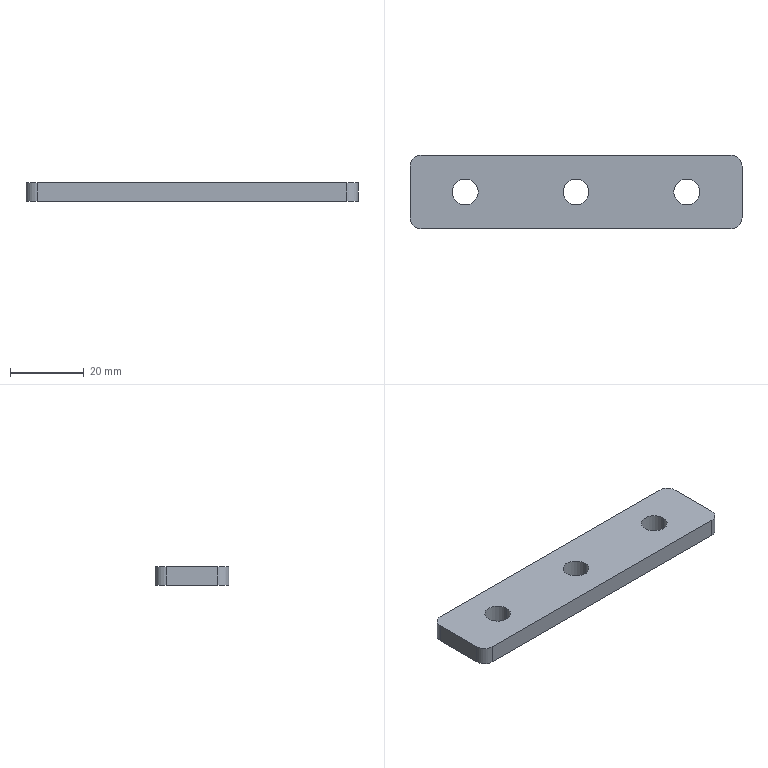Part | SolidWorks | features BaseBody 1 | 1 solid | 16 faces | box 90 x 20 x 5 mm | volume 8384 mm3 | cylinder 10 | plane 6 | commonest cylinder face diameters 7 x6 6 x4
STEP:
#1=CARTESIAN_POINT('',(26.5,0.,5.));
#2=VERTEX_POINT('',#1);
#3=CARTESIAN_POINT('',(33.5,0.,5.));
#4=VERTEX_POINT('',#3);
#5=CARTESIAN_POINT('',(30.,0.,5.));
#6=DIRECTION('',(0.,0.,1.));
#7=DIRECTION('',(1.,0.,0.));
#8=AXIS2_PLACEMENT_3D('',#5,#6,#7);
#9=CIRCLE('',#8,3.5);
#10=EDGE_CURVE('',#2,#4,#9,.T.);
#11=ORIENTED_EDGE('',*,*,#10,.T.);
#12=CARTESIAN_POINT('',(33.5,0.,0.));
#13=VERTEX_POINT('',#12);
#14=CARTESIAN_POINT('',(33.5,0.,5.));
#15=DIRECTION('',(0.,0.,-1.));
#16=VECTOR('',#15,1000.);
#17=LINE('',#14,#16);
#18=EDGE_CURVE('',#4,#13,#17,.T.);
#19=ORIENTED_EDGE('',*,*,#18,.T.);
#20=CARTESIAN_POINT('',(26.5,0.,0.));
#21=VERTEX_POINT('',#20);
#22=CARTESIAN_POINT('',(30.,0.,0.));
#23=DIRECTION('',(0.,0.,1.));
#24=DIRECTION('',(1.,0.,0.));
#25=AXIS2_PLACEMENT_3D('',#22,#23,#24);
#26=CIRCLE('',#25,3.5);
#27=EDGE_CURVE('',#21,#13,#26,.T.);
#28=ORIENTED_EDGE('',*,*,#27,.F.);
#29=CARTESIAN_POINT('',(26.5,0.,5.));
#30=DIRECTION('',(0.,0.,-1.));
#31=VECTOR('',#30,1000.);
#32=LINE('',#29,#31);
#33=EDGE_CURVE('',#2,#21,#32,.T.);
#34=ORIENTED_EDGE('',*,*,#33,.F.);
#35=EDGE_LOOP('',(#11,#19,#28,#34));
#36=FACE_OUTER_BOUND('',#35,.T.);
#37=CARTESIAN_POINT('',(30.,0.,5.));
#38=DIRECTION('',(0.,0.,-1.));
#39=DIRECTION('',(-1.,0.,0.));
#40=AXIS2_PLACEMENT_3D('',#37,#38,#39);
#41=CYLINDRICAL_SURFACE('',#40,3.5);
#42=ADVANCED_FACE('',(#36),#41,.F.);
#43=CARTESIAN_POINT('',(-3.5,0.,5.));
#44=VERTEX_POINT('',#43);
#45=CARTESIAN_POINT('',(3.5,0.,5.));
#46=VERTEX_POINT('',#45);
#47=CARTESIAN_POINT('',(0.,0.,5.));
#48=DIRECTION('',(0.,0.,1.));
#49=DIRECTION('',(-1.,0.,0.));
#50=AXIS2_PLACEMENT_3D('',#47,#48,#49);
#51=CIRCLE('',#50,3.5);
#52=EDGE_CURVE('',#44,#46,#51,.T.);
#53=ORIENTED_EDGE('',*,*,#52,.T.);
#54=CARTESIAN_POINT('',(3.5,0.,0.));
#55=VERTEX_POINT('',#54);
#56=CARTESIAN_POINT('',(3.5,0.,5.));
#57=DIRECTION('',(0.,0.,-1.));
#58=VECTOR('',#57,1000.);
#59=LINE('',#56,#58);
#60=EDGE_CURVE('',#46,#55,#59,.T.);
#61=ORIENTED_EDGE('',*,*,#60,.T.);
#62=CARTESIAN_POINT('',(-3.5,0.,0.));
#63=VERTEX_POINT('',#62);
#64=CARTESIAN_POINT('',(0.,0.,0.));
#65=DIRECTION('',(0.,0.,1.));
#66=DIRECTION('',(-1.,0.,0.));
#67=AXIS2_PLACEMENT_3D('',#64,#65,#66);
#68=CIRCLE('',#67,3.5);
#69=EDGE_CURVE('',#63,#55,#68,.T.);
#70=ORIENTED_EDGE('',*,*,#69,.F.);
#71=CARTESIAN_POINT('',(-3.5,0.,5.));
#72=DIRECTION('',(0.,0.,-1.));
#73=VECTOR('',#72,1000.);
#74=LINE('',#71,#73);
#75=EDGE_CURVE('',#44,#63,#74,.T.);
#76=ORIENTED_EDGE('',*,*,#75,.F.);
#77=EDGE_LOOP('',(#53,#61,#70,#76));
#78=FACE_OUTER_BOUND('',#77,.T.);
#79=CARTESIAN_POINT('',(0.,0.,5.));
#80=DIRECTION('',(0.,0.,-1.));
#81=DIRECTION('',(-1.,0.,0.));
#82=AXIS2_PLACEMENT_3D('',#79,#80,#81);
#83=CYLINDRICAL_SURFACE('',#82,3.5);
#84=ADVANCED_FACE('',(#78),#83,.F.);
#85=CARTESIAN_POINT('',(-33.5,0.,5.));
#86=VERTEX_POINT('',#85);
#87=CARTESIAN_POINT('',(-26.5,0.,5.));
#88=VERTEX_POINT('',#87);
#89=CARTESIAN_POINT('',(-30.,0.,5.));
#90=DIRECTION('',(0.,0.,1.));
#91=DIRECTION('',(1.,0.,0.));
#92=AXIS2_PLACEMENT_3D('',#89,#90,#91);
#93=CIRCLE('',#92,3.5);
#94=EDGE_CURVE('',#86,#88,#93,.T.);
#95=ORIENTED_EDGE('',*,*,#94,.T.);
#96=CARTESIAN_POINT('',(-26.5,0.,0.));
#97=VERTEX_POINT('',#96);
#98=CARTESIAN_POINT('',(-26.5,0.,5.));
#99=DIRECTION('',(0.,0.,-1.));
#100=VECTOR('',#99,1000.);
#101=LINE('',#98,#100);
#102=EDGE_CURVE('',#88,#97,#101,.T.);
#103=ORIENTED_EDGE('',*,*,#102,.T.);
#104=CARTESIAN_POINT('',(-33.5,0.,0.));
#105=VERTEX_POINT('',#104);
#106=CARTESIAN_POINT('',(-30.,0.,0.));
#107=DIRECTION('',(0.,0.,1.));
#108=DIRECTION('',(1.,0.,0.));
#109=AXIS2_PLACEMENT_3D('',#106,#107,#108);
#110=CIRCLE('',#109,3.5);
#111=EDGE_CURVE('',#105,#97,#110,.T.);
#112=ORIENTED_EDGE('',*,*,#111,.F.);
#113=CARTESIAN_POINT('',(-33.5,0.,5.));
#114=DIRECTION('',(0.,0.,-1.));
#115=VECTOR('',#114,1000.);
#116=LINE('',#113,#115);
#117=EDGE_CURVE('',#86,#105,#116,.T.);
#118=ORIENTED_EDGE('',*,*,#117,.F.);
#119=EDGE_LOOP('',(#95,#103,#112,#118));
#120=FACE_OUTER_BOUND('',#119,.T.);
#121=CARTESIAN_POINT('',(-30.,0.,5.));
#122=DIRECTION('',(0.,0.,-1.));
#123=DIRECTION('',(-1.,0.,0.));
#124=AXIS2_PLACEMENT_3D('',#121,#122,#123);
#125=CYLINDRICAL_SURFACE('',#124,3.5);
#126=ADVANCED_FACE('',(#120),#125,.F.);
#127=CARTESIAN_POINT('',(-45.,7.,5.));
#128=VERTEX_POINT('',#127);
#129=CARTESIAN_POINT('',(-45.,-7.,5.));
#130=VERTEX_POINT('',#129);
#131=CARTESIAN_POINT('',(-45.,-10.,5.));
#132=DIRECTION('',(0.,-1.,0.));
#133=VECTOR('',#132,1000.);
#134=LINE('',#131,#133);
#135=EDGE_CURVE('',#128,#130,#134,.T.);
#136=ORIENTED_EDGE('',*,*,#135,.T.);
#137=CARTESIAN_POINT('',(-42.,-10.,5.));
#138=VERTEX_POINT('',#137);
#139=CARTESIAN_POINT('',(-42.,-7.,5.));
#140=DIRECTION('',(0.,0.,1.));
#141=DIRECTION('',(-1.,0.,0.));
#142=AXIS2_PLACEMENT_3D('',#139,#140,#141);
#143=CIRCLE('',#142,3.);
#144=EDGE_CURVE('',#130,#138,#143,.T.);
#145=ORIENTED_EDGE('',*,*,#144,.T.);
#146=CARTESIAN_POINT('',(42.,-10.,5.));
#147=VERTEX_POINT('',#146);
#148=CARTESIAN_POINT('',(-45.,-10.,5.));
#149=DIRECTION('',(1.,0.,0.));
#150=VECTOR('',#149,1000.);
#151=LINE('',#148,#150);
#152=EDGE_CURVE('',#138,#147,#151,.T.);
#153=ORIENTED_EDGE('',*,*,#152,.T.);
#154=CARTESIAN_POINT('',(45.,-7.,5.));
#155=VERTEX_POINT('',#154);
#156=CARTESIAN_POINT('',(42.,-7.,5.));
#157=DIRECTION('',(0.,0.,1.));
#158=DIRECTION('',(-1.,0.,0.));
#159=AXIS2_PLACEMENT_3D('',#156,#157,#158);
#160=CIRCLE('',#159,3.);
#161=EDGE_CURVE('',#147,#155,#160,.T.);
#162=ORIENTED_EDGE('',*,*,#161,.T.);
#163=CARTESIAN_POINT('',(45.,7.,5.));
#164=VERTEX_POINT('',#163);
#165=CARTESIAN_POINT('',(45.,-10.,5.));
#166=DIRECTION('',(0.,1.,0.));
#167=VECTOR('',#166,1000.);
#168=LINE('',#165,#167);
#169=EDGE_CURVE('',#155,#164,#168,.T.);
#170=ORIENTED_EDGE('',*,*,#169,.T.);
#171=CARTESIAN_POINT('',(42.,10.,5.));
#172=VERTEX_POINT('',#171);
#173=CARTESIAN_POINT('',(42.,7.,5.));
#174=DIRECTION('',(0.,0.,1.));
#175=DIRECTION('',(-1.,0.,0.));
#176=AXIS2_PLACEMENT_3D('',#173,#174,#175);
#177=CIRCLE('',#176,3.);
#178=EDGE_CURVE('',#164,#172,#177,.T.);
#179=ORIENTED_EDGE('',*,*,#178,.T.);
#180=CARTESIAN_POINT('',(-42.,10.,5.));
#181=VERTEX_POINT('',#180);
#182=CARTESIAN_POINT('',(-45.,10.,5.));
#183=DIRECTION('',(-1.,0.,0.));
#184=VECTOR('',#183,1000.);
#185=LINE('',#182,#184);
#186=EDGE_CURVE('',#172,#181,#185,.T.);
#187=ORIENTED_EDGE('',*,*,#186,.T.);
#188=CARTESIAN_POINT('',(-42.,7.,5.));
#189=DIRECTION('',(0.,0.,1.));
#190=DIRECTION('',(-1.,0.,0.));
#191=AXIS2_PLACEMENT_3D('',#188,#189,#190);
#192=CIRCLE('',#191,3.);
#193=EDGE_CURVE('',#181,#128,#192,.T.);
#194=ORIENTED_EDGE('',*,*,#193,.T.);
#195=EDGE_LOOP('',(#136,#145,#153,#162,#170,#179,#187,#194));
#196=FACE_OUTER_BOUND('',#195,.T.);
#197=ORIENTED_EDGE('',*,*,#94,.F.);
#198=CARTESIAN_POINT('',(-30.,0.,5.));
#199=DIRECTION('',(0.,0.,1.));
#200=DIRECTION('',(1.,0.,0.));
#201=AXIS2_PLACEMENT_3D('',#198,#199,#200);
#202=CIRCLE('',#201,3.5);
#203=EDGE_CURVE('',#88,#86,#202,.T.);
#204=ORIENTED_EDGE('',*,*,#203,.F.);
#205=EDGE_LOOP('',(#197,#204));
#206=FACE_BOUND('',#205,.T.);
#207=ORIENTED_EDGE('',*,*,#52,.F.);
#208=CARTESIAN_POINT('',(0.,0.,5.));
#209=DIRECTION('',(0.,0.,1.));
#210=DIRECTION('',(-1.,0.,0.));
#211=AXIS2_PLACEMENT_3D('',#208,#209,#210);
#212=CIRCLE('',#211,3.5);
#213=EDGE_CURVE('',#46,#44,#212,.T.);
#214=ORIENTED_EDGE('',*,*,#213,.F.);
#215=EDGE_LOOP('',(#207,#214));
#216=FACE_BOUND('',#215,.T.);
#217=ORIENTED_EDGE('',*,*,#10,.F.);
#218=CARTESIAN_POINT('',(30.,0.,5.));
#219=DIRECTION('',(0.,0.,1.));
#220=DIRECTION('',(1.,0.,0.));
#221=AXIS2_PLACEMENT_3D('',#218,#219,#220);
#222=CIRCLE('',#221,3.5);
#223=EDGE_CURVE('',#4,#2,#222,.T.);
#224=ORIENTED_EDGE('',*,*,#223,.F.);
#225=EDGE_LOOP('',(#217,#224));
#226=FACE_BOUND('',#225,.T.);
#227=CARTESIAN_POINT('',(0.,0.,5.));
#228=DIRECTION('',(0.,0.,-1.));
#229=DIRECTION('',(-1.,0.,0.));
#230=AXIS2_PLACEMENT_3D('',#227,#228,#229);
#231=PLANE('',#230);
#232=ADVANCED_FACE('',(#196,#206,#216,#226),#231,.F.);
#233=ORIENTED_EDGE('',*,*,#69,.T.);
#234=CARTESIAN_POINT('',(0.,0.,0.));
#235=DIRECTION('',(0.,0.,1.));
#236=DIRECTION('',(-1.,0.,0.));
#237=AXIS2_PLACEMENT_3D('',#234,#235,#236);
#238=CIRCLE('',#237,3.5);
#239=EDGE_CURVE('',#55,#63,#238,.T.);
#240=ORIENTED_EDGE('',*,*,#239,.T.);
#241=EDGE_LOOP('',(#233,#240));
#242=FACE_BOUND('',#241,.T.);
#243=CARTESIAN_POINT('',(-42.,-10.,0.));
#244=VERTEX_POINT('',#243);
#245=CARTESIAN_POINT('',(42.,-10.,0.));
#246=VERTEX_POINT('',#245);
#247=CARTESIAN_POINT('',(-45.,-10.,0.));
#248=DIRECTION('',(1.,0.,0.));
#249=VECTOR('',#248,1000.);
#250=LINE('',#247,#249);
#251=EDGE_CURVE('',#244,#246,#250,.T.);
#252=ORIENTED_EDGE('',*,*,#251,.F.);
#253=CARTESIAN_POINT('',(-45.,-7.,0.));
#254=VERTEX_POINT('',#253);
#255=CARTESIAN_POINT('',(-42.,-7.,0.));
#256=DIRECTION('',(0.,0.,-1.));
#257=DIRECTION('',(-1.,0.,0.));
#258=AXIS2_PLACEMENT_3D('',#255,#256,#257);
#259=CIRCLE('',#258,3.);
#260=EDGE_CURVE('',#244,#254,#259,.T.);
#261=ORIENTED_EDGE('',*,*,#260,.T.);
#262=CARTESIAN_POINT('',(-45.,7.,0.));
#263=VERTEX_POINT('',#262);
#264=CARTESIAN_POINT('',(-45.,-10.,0.));
#265=DIRECTION('',(0.,-1.,0.));
#266=VECTOR('',#265,1000.);
#267=LINE('',#264,#266);
#268=EDGE_CURVE('',#263,#254,#267,.T.);
#269=ORIENTED_EDGE('',*,*,#268,.F.);
#270=CARTESIAN_POINT('',(-42.,10.,0.));
#271=VERTEX_POINT('',#270);
#272=CARTESIAN_POINT('',(-42.,7.,0.));
#273=DIRECTION('',(0.,0.,-1.));
#274=DIRECTION('',(-1.,0.,0.));
#275=AXIS2_PLACEMENT_3D('',#272,#273,#274);
#276=CIRCLE('',#275,3.);
#277=EDGE_CURVE('',#263,#271,#276,.T.);
#278=ORIENTED_EDGE('',*,*,#277,.T.);
#279=CARTESIAN_POINT('',(42.,10.,0.));
#280=VERTEX_POINT('',#279);
#281=CARTESIAN_POINT('',(-45.,10.,0.));
#282=DIRECTION('',(-1.,0.,0.));
#283=VECTOR('',#282,1000.);
#284=LINE('',#281,#283);
#285=EDGE_CURVE('',#280,#271,#284,.T.);
#286=ORIENTED_EDGE('',*,*,#285,.F.);
#287=CARTESIAN_POINT('',(45.,7.,0.));
#288=VERTEX_POINT('',#287);
#289=CARTESIAN_POINT('',(42.,7.,0.));
#290=DIRECTION('',(0.,0.,-1.));
#291=DIRECTION('',(-1.,0.,0.));
#292=AXIS2_PLACEMENT_3D('',#289,#290,#291);
#293=CIRCLE('',#292,3.);
#294=EDGE_CURVE('',#280,#288,#293,.T.);
#295=ORIENTED_EDGE('',*,*,#294,.T.);
#296=CARTESIAN_POINT('',(45.,-7.,0.));
#297=VERTEX_POINT('',#296);
#298=CARTESIAN_POINT('',(45.,-10.,0.));
#299=DIRECTION('',(0.,1.,0.));
#300=VECTOR('',#299,1000.);
#301=LINE('',#298,#300);
#302=EDGE_CURVE('',#297,#288,#301,.T.);
#303=ORIENTED_EDGE('',*,*,#302,.F.);
#304=CARTESIAN_POINT('',(42.,-7.,0.));
#305=DIRECTION('',(0.,0.,-1.));
#306=DIRECTION('',(-1.,0.,0.));
#307=AXIS2_PLACEMENT_3D('',#304,#305,#306);
#308=CIRCLE('',#307,3.);
#309=EDGE_CURVE('',#297,#246,#308,.T.);
#310=ORIENTED_EDGE('',*,*,#309,.T.);
#311=EDGE_LOOP('',(#252,#261,#269,#278,#286,#295,#303,#310));
#312=FACE_OUTER_BOUND('',#311,.T.);
#313=ORIENTED_EDGE('',*,*,#111,.T.);
#314=CARTESIAN_POINT('',(-30.,0.,0.));
#315=DIRECTION('',(0.,0.,1.));
#316=DIRECTION('',(1.,0.,0.));
#317=AXIS2_PLACEMENT_3D('',#314,#315,#316);
#318=CIRCLE('',#317,3.5);
#319=EDGE_CURVE('',#97,#105,#318,.T.);
#320=ORIENTED_EDGE('',*,*,#319,.T.);
#321=EDGE_LOOP('',(#313,#320));
#322=FACE_BOUND('',#321,.T.);
#323=ORIENTED_EDGE('',*,*,#27,.T.);
#324=CARTESIAN_POINT('',(30.,0.,0.));
#325=DIRECTION('',(0.,0.,1.));
#326=DIRECTION('',(1.,0.,0.));
#327=AXIS2_PLACEMENT_3D('',#324,#325,#326);
#328=CIRCLE('',#327,3.5);
#329=EDGE_CURVE('',#13,#21,#328,.T.);
#330=ORIENTED_EDGE('',*,*,#329,.T.);
#331=EDGE_LOOP('',(#323,#330));
#332=FACE_BOUND('',#331,.T.);
#333=CARTESIAN_POINT('',(0.,0.,0.));
#334=DIRECTION('',(0.,0.,-1.));
#335=DIRECTION('',(-1.,0.,0.));
#336=AXIS2_PLACEMENT_3D('',#333,#334,#335);
#337=PLANE('',#336);
#338=ADVANCED_FACE('',(#242,#312,#322,#332),#337,.T.);
#339=ORIENTED_EDGE('',*,*,#169,.F.);
#340=CARTESIAN_POINT('',(45.,-7.,5.));
#341=DIRECTION('',(0.,0.,-1.));
#342=VECTOR('',#341,1000.);
#343=LINE('',#340,#342);
#344=EDGE_CURVE('',#155,#297,#343,.T.);
#345=ORIENTED_EDGE('',*,*,#344,.T.);
#346=ORIENTED_EDGE('',*,*,#302,.T.);
#347=CARTESIAN_POINT('',(45.,7.,5.));
#348=DIRECTION('',(0.,0.,1.));
#349=VECTOR('',#348,1000.);
#350=LINE('',#347,#349);
#351=EDGE_CURVE('',#288,#164,#350,.T.);
#352=ORIENTED_EDGE('',*,*,#351,.T.);
#353=EDGE_LOOP('',(#339,#345,#346,#352));
#354=FACE_OUTER_BOUND('',#353,.T.);
#355=CARTESIAN_POINT('',(45.,-10.,5.));
#356=DIRECTION('',(-1.,0.,0.));
#357=DIRECTION('',(0.,-1.,0.));
#358=AXIS2_PLACEMENT_3D('',#355,#356,#357);
#359=PLANE('',#358);
#360=ADVANCED_FACE('',(#354),#359,.F.);
#361=ORIENTED_EDGE('',*,*,#186,.F.);
#362=CARTESIAN_POINT('',(42.,10.,5.));
#363=DIRECTION('',(0.,0.,-1.));
#364=VECTOR('',#363,1000.);
#365=LINE('',#362,#364);
#366=EDGE_CURVE('',#172,#280,#365,.T.);
#367=ORIENTED_EDGE('',*,*,#366,.T.);
#368=ORIENTED_EDGE('',*,*,#285,.T.);
#369=CARTESIAN_POINT('',(-42.,10.,5.));
#370=DIRECTION('',(0.,0.,1.));
#371=VECTOR('',#370,1000.);
#372=LINE('',#369,#371);
#373=EDGE_CURVE('',#271,#181,#372,.T.);
#374=ORIENTED_EDGE('',*,*,#373,.T.);
#375=EDGE_LOOP('',(#361,#367,#368,#374));
#376=FACE_OUTER_BOUND('',#375,.T.);
#377=CARTESIAN_POINT('',(-45.,10.,5.));
#378=DIRECTION('',(0.,-1.,0.));
#379=DIRECTION('',(1.,0.,0.));
#380=AXIS2_PLACEMENT_3D('',#377,#378,#379);
#381=PLANE('',#380);
#382=ADVANCED_FACE('',(#376),#381,.F.);
#383=ORIENTED_EDGE('',*,*,#268,.T.);
#384=CARTESIAN_POINT('',(-45.,-7.,5.));
#385=DIRECTION('',(0.,0.,1.));
#386=VECTOR('',#385,1000.);
#387=LINE('',#384,#386);
#388=EDGE_CURVE('',#254,#130,#387,.T.);
#389=ORIENTED_EDGE('',*,*,#388,.T.);
#390=ORIENTED_EDGE('',*,*,#135,.F.);
#391=CARTESIAN_POINT('',(-45.,7.,5.));
#392=DIRECTION('',(0.,0.,-1.));
#393=VECTOR('',#392,1000.);
#394=LINE('',#391,#393);
#395=EDGE_CURVE('',#128,#263,#394,.T.);
#396=ORIENTED_EDGE('',*,*,#395,.T.);
#397=EDGE_LOOP('',(#383,#389,#390,#396));
#398=FACE_OUTER_BOUND('',#397,.T.);
#399=CARTESIAN_POINT('',(-45.,-10.,5.));
#400=DIRECTION('',(1.,0.,0.));
#401=DIRECTION('',(0.,0.,-1.));
#402=AXIS2_PLACEMENT_3D('',#399,#400,#401);
#403=PLANE('',#402);
#404=ADVANCED_FACE('',(#398),#403,.F.);
#405=ORIENTED_EDGE('',*,*,#152,.F.);
#406=CARTESIAN_POINT('',(-42.,-10.,5.));
#407=DIRECTION('',(0.,0.,-1.));
#408=VECTOR('',#407,1000.);
#409=LINE('',#406,#408);
#410=EDGE_CURVE('',#138,#244,#409,.T.);
#411=ORIENTED_EDGE('',*,*,#410,.T.);
#412=ORIENTED_EDGE('',*,*,#251,.T.);
#413=CARTESIAN_POINT('',(42.,-10.,5.));
#414=DIRECTION('',(0.,0.,1.));
#415=VECTOR('',#414,1000.);
#416=LINE('',#413,#415);
#417=EDGE_CURVE('',#246,#147,#416,.T.);
#418=ORIENTED_EDGE('',*,*,#417,.T.);
#419=EDGE_LOOP('',(#405,#411,#412,#418));
#420=FACE_OUTER_BOUND('',#419,.T.);
#421=CARTESIAN_POINT('',(-45.,-10.,5.));
#422=DIRECTION('',(0.,1.,0.));
#423=DIRECTION('',(-1.,0.,0.));
#424=AXIS2_PLACEMENT_3D('',#421,#422,#423);
#425=PLANE('',#424);
#426=ADVANCED_FACE('',(#420),#425,.F.);
#427=ORIENTED_EDGE('',*,*,#102,.F.);
#428=ORIENTED_EDGE('',*,*,#203,.T.);
#429=ORIENTED_EDGE('',*,*,#117,.T.);
#430=ORIENTED_EDGE('',*,*,#319,.F.);
#431=EDGE_LOOP('',(#427,#428,#429,#430));
#432=FACE_OUTER_BOUND('',#431,.T.);
#433=CARTESIAN_POINT('',(-30.,0.,5.));
#434=DIRECTION('',(0.,0.,-1.));
#435=DIRECTION('',(-1.,0.,0.));
#436=AXIS2_PLACEMENT_3D('',#433,#434,#435);
#437=CYLINDRICAL_SURFACE('',#436,3.5);
#438=ADVANCED_FACE('',(#432),#437,.F.);
#439=ORIENTED_EDGE('',*,*,#60,.F.);
#440=ORIENTED_EDGE('',*,*,#213,.T.);
#441=ORIENTED_EDGE('',*,*,#75,.T.);
#442=ORIENTED_EDGE('',*,*,#239,.F.);
#443=EDGE_LOOP('',(#439,#440,#441,#442));
#444=FACE_OUTER_BOUND('',#443,.T.);
#445=CARTESIAN_POINT('',(0.,0.,5.));
#446=DIRECTION('',(0.,0.,-1.));
#447=DIRECTION('',(-1.,0.,0.));
#448=AXIS2_PLACEMENT_3D('',#445,#446,#447);
#449=CYLINDRICAL_SURFACE('',#448,3.5);
#450=ADVANCED_FACE('',(#444),#449,.F.);
#451=ORIENTED_EDGE('',*,*,#18,.F.);
#452=ORIENTED_EDGE('',*,*,#223,.T.);
#453=ORIENTED_EDGE('',*,*,#33,.T.);
#454=ORIENTED_EDGE('',*,*,#329,.F.);
#455=EDGE_LOOP('',(#451,#452,#453,#454));
#456=FACE_OUTER_BOUND('',#455,.T.);
#457=CARTESIAN_POINT('',(30.,0.,5.));
#458=DIRECTION('',(0.,0.,-1.));
#459=DIRECTION('',(-1.,0.,0.));
#460=AXIS2_PLACEMENT_3D('',#457,#458,#459);
#461=CYLINDRICAL_SURFACE('',#460,3.5);
#462=ADVANCED_FACE('',(#456),#461,.F.);
#463=ORIENTED_EDGE('',*,*,#144,.F.);
#464=ORIENTED_EDGE('',*,*,#388,.F.);
#465=ORIENTED_EDGE('',*,*,#260,.F.);
#466=ORIENTED_EDGE('',*,*,#410,.F.);
#467=EDGE_LOOP('',(#463,#464,#465,#466));
#468=FACE_OUTER_BOUND('',#467,.T.);
#469=CARTESIAN_POINT('',(-42.,-7.,5.));
#470=DIRECTION('',(0.,0.,-1.));
#471=DIRECTION('',(-1.,0.,0.));
#472=AXIS2_PLACEMENT_3D('',#469,#470,#471);
#473=CYLINDRICAL_SURFACE('',#472,3.);
#474=ADVANCED_FACE('',(#468),#473,.T.);
#475=ORIENTED_EDGE('',*,*,#161,.F.);
#476=ORIENTED_EDGE('',*,*,#417,.F.);
#477=ORIENTED_EDGE('',*,*,#309,.F.);
#478=ORIENTED_EDGE('',*,*,#344,.F.);
#479=EDGE_LOOP('',(#475,#476,#477,#478));
#480=FACE_OUTER_BOUND('',#479,.T.);
#481=CARTESIAN_POINT('',(42.,-7.,5.));
#482=DIRECTION('',(0.,0.,-1.));
#483=DIRECTION('',(-1.,0.,0.));
#484=AXIS2_PLACEMENT_3D('',#481,#482,#483);
#485=CYLINDRICAL_SURFACE('',#484,3.);
#486=ADVANCED_FACE('',(#480),#485,.T.);
#487=ORIENTED_EDGE('',*,*,#178,.F.);
#488=ORIENTED_EDGE('',*,*,#351,.F.);
#489=ORIENTED_EDGE('',*,*,#294,.F.);
#490=ORIENTED_EDGE('',*,*,#366,.F.);
#491=EDGE_LOOP('',(#487,#488,#489,#490));
#492=FACE_OUTER_BOUND('',#491,.T.);
#493=CARTESIAN_POINT('',(42.,7.,5.));
#494=DIRECTION('',(0.,0.,-1.));
#495=DIRECTION('',(-1.,0.,0.));
#496=AXIS2_PLACEMENT_3D('',#493,#494,#495);
#497=CYLINDRICAL_SURFACE('',#496,3.);
#498=ADVANCED_FACE('',(#492),#497,.T.);
#499=ORIENTED_EDGE('',*,*,#193,.F.);
#500=ORIENTED_EDGE('',*,*,#373,.F.);
#501=ORIENTED_EDGE('',*,*,#277,.F.);
#502=ORIENTED_EDGE('',*,*,#395,.F.);
#503=EDGE_LOOP('',(#499,#500,#501,#502));
#504=FACE_OUTER_BOUND('',#503,.T.);
#505=CARTESIAN_POINT('',(-42.,7.,5.));
#506=DIRECTION('',(0.,0.,-1.));
#507=DIRECTION('',(-1.,0.,0.));
#508=AXIS2_PLACEMENT_3D('',#505,#506,#507);
#509=CYLINDRICAL_SURFACE('',#508,3.);
#510=ADVANCED_FACE('',(#504),#509,.T.);
#511=CLOSED_SHELL('',(#42,#84,#126,#232,#338,#360,#382,#404,#426,#438,#450,#462,#474,#486,#498,#510));
#512=MANIFOLD_SOLID_BREP('',#511);
#513=CARTESIAN_POINT('',(0.,0.,0.));
#514=DIRECTION('',(0.,0.,1.));
#515=DIRECTION('',(1.,0.,0.));
#516=AXIS2_PLACEMENT_3D('',#513,#514,#515);
#517=(LENGTH_UNIT()NAMED_UNIT(*)SI_UNIT(.MILLI.,.METRE.));
#518=UNCERTAINTY_MEASURE_WITH_UNIT(LENGTH_MEASURE(0.00001),#517,'','');
#519=(NAMED_UNIT(*)PLANE_ANGLE_UNIT()SI_UNIT($,.RADIAN.));
#520=(NAMED_UNIT(*)SI_UNIT($,.STERADIAN.)SOLID_ANGLE_UNIT());
#521=(GEOMETRIC_REPRESENTATION_CONTEXT(3)GLOBAL_UNCERTAINTY_ASSIGNED_CONTEXT((#518))GLOBAL_UNIT_ASSIGNED_CONTEXT((#517,#519,#520))REPRESENTATION_CONTEXT('',''));
#522=ADVANCED_BREP_SHAPE_REPRESENTATION('',(#512,#516),#521);